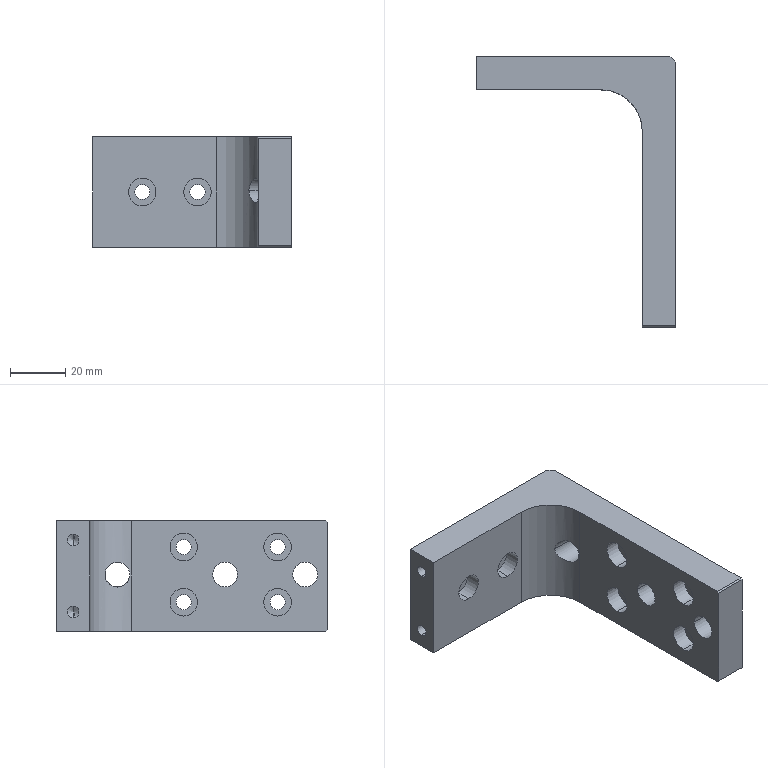Part | SolidWorks | features HoleWzd 3, Chamfer 2, Cut 1, Extrusion 1, Fillet 1 | 1 solid | 56 faces | box 72 x 98 x 40 mm | volume 71413 mm3 | cylinder 35 | plane 17 | cone 4 | commonest cylinder face diameters 5.5 x12 10 x12 9 x6 4.2 x4 30 x1